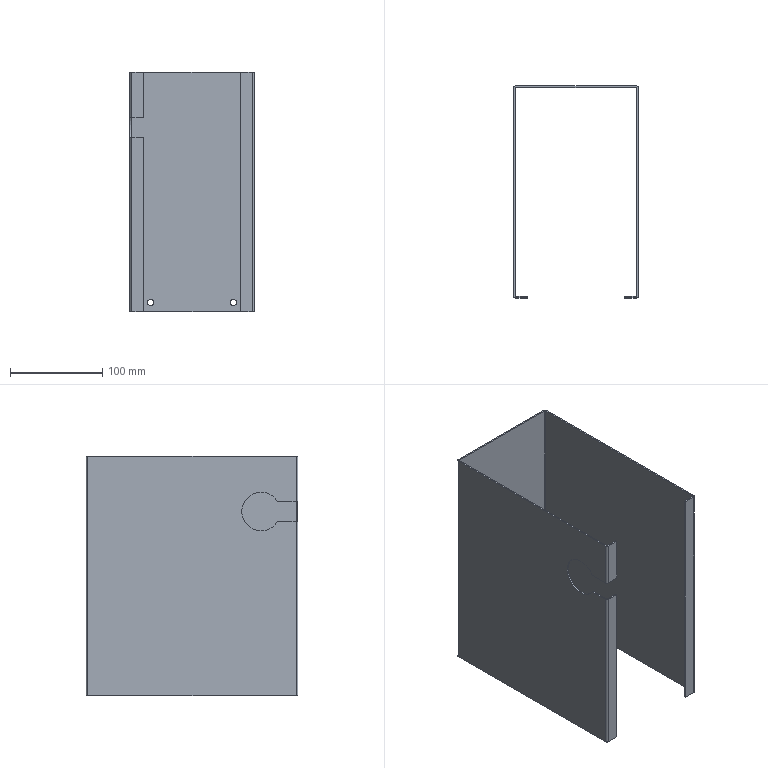Part | STEP file | X Motor Cover 1 | 1 solid | 36 faces | box 135 x 230 x 260 mm | volume 237291 mm3 | plane 19 | cylinder 17 | commonest cylinder face diameters 1 x5 4 x5 7 x4 42 x3
STEP:
#1=CARTESIAN_POINT('',(-74.708,228.5,-161.347));
#2=VERTEX_POINT('',#1);
#3=CARTESIAN_POINT('',(-74.708,228.5,-168.347));
#4=VERTEX_POINT('',#3);
#5=CARTESIAN_POINT('',(-74.708,228.5,-164.847));
#6=DIRECTION('',(0.,-1.,0.));
#7=DIRECTION('',(0.,0.,1.));
#8=AXIS2_PLACEMENT_3D('',#5,#6,#7);
#9=CIRCLE('',#8,3.5);
#10=EDGE_CURVE('',#2,#4,#9,.T.);
#11=ORIENTED_EDGE('',*,*,#10,.T.);
#12=CARTESIAN_POINT('',(-74.708,230.,-168.347));
#13=VERTEX_POINT('',#12);
#14=CARTESIAN_POINT('',(-74.708,208.,-168.347));
#15=DIRECTION('',(0.,1.,0.));
#16=VECTOR('',#15,1000.);
#17=LINE('',#14,#16);
#18=EDGE_CURVE('',#4,#13,#17,.T.);
#19=ORIENTED_EDGE('',*,*,#18,.T.);
#20=CARTESIAN_POINT('',(-74.708,230.,-161.347));
#21=VERTEX_POINT('',#20);
#22=CARTESIAN_POINT('',(-74.708,230.,-164.847));
#23=DIRECTION('',(0.,-1.,0.));
#24=DIRECTION('',(0.,0.,1.));
#25=AXIS2_PLACEMENT_3D('',#22,#23,#24);
#26=CIRCLE('',#25,3.5);
#27=EDGE_CURVE('',#21,#13,#26,.T.);
#28=ORIENTED_EDGE('',*,*,#27,.F.);
#29=CARTESIAN_POINT('',(-74.708,208.,-161.347));
#30=DIRECTION('',(0.,1.,0.));
#31=VECTOR('',#30,1000.);
#32=LINE('',#29,#31);
#33=EDGE_CURVE('',#2,#21,#32,.T.);
#34=ORIENTED_EDGE('',*,*,#33,.F.);
#35=EDGE_LOOP('',(#11,#19,#28,#34));
#36=FACE_OUTER_BOUND('',#35,.T.);
#37=CARTESIAN_POINT('',(-74.708,208.,-164.847));
#38=DIRECTION('',(0.,1.,0.));
#39=DIRECTION('',(0.,0.,1.));
#40=AXIS2_PLACEMENT_3D('',#37,#38,#39);
#41=CYLINDRICAL_SURFACE('',#40,3.5);
#42=ADVANCED_FACE('',(#36),#41,.F.);
#43=CARTESIAN_POINT('',(15.292,228.5,-161.347));
#44=VERTEX_POINT('',#43);
#45=CARTESIAN_POINT('',(15.292,228.5,-168.347));
#46=VERTEX_POINT('',#45);
#47=CARTESIAN_POINT('',(15.292,228.5,-164.847));
#48=DIRECTION('',(0.,-1.,0.));
#49=DIRECTION('',(0.,0.,1.));
#50=AXIS2_PLACEMENT_3D('',#47,#48,#49);
#51=CIRCLE('',#50,3.5);
#52=EDGE_CURVE('',#44,#46,#51,.T.);
#53=ORIENTED_EDGE('',*,*,#52,.T.);
#54=CARTESIAN_POINT('',(15.292,230.,-168.347));
#55=VERTEX_POINT('',#54);
#56=CARTESIAN_POINT('',(15.292,208.,-168.347));
#57=DIRECTION('',(0.,1.,0.));
#58=VECTOR('',#57,1000.);
#59=LINE('',#56,#58);
#60=EDGE_CURVE('',#46,#55,#59,.T.);
#61=ORIENTED_EDGE('',*,*,#60,.T.);
#62=CARTESIAN_POINT('',(15.292,230.,-161.347));
#63=VERTEX_POINT('',#62);
#64=CARTESIAN_POINT('',(15.292,230.,-164.847));
#65=DIRECTION('',(0.,-1.,0.));
#66=DIRECTION('',(0.,0.,1.));
#67=AXIS2_PLACEMENT_3D('',#64,#65,#66);
#68=CIRCLE('',#67,3.5);
#69=EDGE_CURVE('',#63,#55,#68,.T.);
#70=ORIENTED_EDGE('',*,*,#69,.F.);
#71=CARTESIAN_POINT('',(15.292,208.,-161.347));
#72=DIRECTION('',(0.,1.,0.));
#73=VECTOR('',#72,1000.);
#74=LINE('',#71,#73);
#75=EDGE_CURVE('',#44,#63,#74,.T.);
#76=ORIENTED_EDGE('',*,*,#75,.F.);
#77=EDGE_LOOP('',(#53,#61,#70,#76));
#78=FACE_OUTER_BOUND('',#77,.T.);
#79=CARTESIAN_POINT('',(15.292,208.,-164.847));
#80=DIRECTION('',(0.,1.,0.));
#81=DIRECTION('',(0.,0.,1.));
#82=AXIS2_PLACEMENT_3D('',#79,#80,#81);
#83=CYLINDRICAL_SURFACE('',#82,3.5);
#84=ADVANCED_FACE('',(#78),#83,.F.);
#85=CARTESIAN_POINT('',(-95.708,40.,4.153));
#86=VERTEX_POINT('',#85);
#87=CARTESIAN_POINT('',(-95.708,22.111,14.153));
#88=VERTEX_POINT('',#87);
#89=CARTESIAN_POINT('',(-95.708,40.,25.153));
#90=DIRECTION('',(-1.,0.,0.));
#91=DIRECTION('',(0.,0.,1.));
#92=AXIS2_PLACEMENT_3D('',#89,#90,#91);
#93=CIRCLE('',#92,21.);
#94=EDGE_CURVE('',#86,#88,#93,.T.);
#95=ORIENTED_EDGE('',*,*,#94,.F.);
#96=CARTESIAN_POINT('',(-97.208,40.,4.153));
#97=VERTEX_POINT('',#96);
#98=CARTESIAN_POINT('',(-75.208,40.,4.153));
#99=DIRECTION('',(-1.,0.,0.));
#100=VECTOR('',#99,1000.);
#101=LINE('',#98,#100);
#102=EDGE_CURVE('',#86,#97,#101,.T.);
#103=ORIENTED_EDGE('',*,*,#102,.T.);
#104=CARTESIAN_POINT('',(-97.208,22.111,14.153));
#105=VERTEX_POINT('',#104);
#106=CARTESIAN_POINT('',(-97.208,40.,25.153));
#107=DIRECTION('',(1.,0.,0.));
#108=DIRECTION('',(0.,0.,1.));
#109=AXIS2_PLACEMENT_3D('',#106,#107,#108);
#110=CIRCLE('',#109,21.);
#111=EDGE_CURVE('',#105,#97,#110,.T.);
#112=ORIENTED_EDGE('',*,*,#111,.F.);
#113=CARTESIAN_POINT('',(-75.208,22.111,14.153));
#114=DIRECTION('',(1.,0.,0.));
#115=VECTOR('',#114,1000.);
#116=LINE('',#113,#115);
#117=EDGE_CURVE('',#105,#88,#116,.T.);
#118=ORIENTED_EDGE('',*,*,#117,.T.);
#119=EDGE_LOOP('',(#95,#103,#112,#118));
#120=FACE_OUTER_BOUND('',#119,.T.);
#121=CARTESIAN_POINT('',(-75.208,40.,25.153));
#122=DIRECTION('',(-1.,0.,0.));
#123=DIRECTION('',(0.,0.,1.));
#124=AXIS2_PLACEMENT_3D('',#121,#122,#123);
#125=CYLINDRICAL_SURFACE('',#124,21.);
#126=ADVANCED_FACE('',(#120),#125,.F.);
#127=ORIENTED_EDGE('',*,*,#102,.F.);
#128=CARTESIAN_POINT('',(-95.708,40.,46.153));
#129=VERTEX_POINT('',#128);
#130=CARTESIAN_POINT('',(-95.708,40.,25.153));
#131=DIRECTION('',(-1.,0.,0.));
#132=DIRECTION('',(0.,0.,1.));
#133=AXIS2_PLACEMENT_3D('',#130,#131,#132);
#134=CIRCLE('',#133,21.);
#135=EDGE_CURVE('',#129,#86,#134,.T.);
#136=ORIENTED_EDGE('',*,*,#135,.F.);
#137=CARTESIAN_POINT('',(-97.208,40.,46.153));
#138=VERTEX_POINT('',#137);
#139=CARTESIAN_POINT('',(-75.208,40.,46.153));
#140=DIRECTION('',(-1.,0.,0.));
#141=VECTOR('',#140,1000.);
#142=LINE('',#139,#141);
#143=EDGE_CURVE('',#129,#138,#142,.T.);
#144=ORIENTED_EDGE('',*,*,#143,.T.);
#145=CARTESIAN_POINT('',(-97.208,40.,25.153));
#146=DIRECTION('',(1.,0.,0.));
#147=DIRECTION('',(0.,0.,1.));
#148=AXIS2_PLACEMENT_3D('',#145,#146,#147);
#149=CIRCLE('',#148,21.);
#150=EDGE_CURVE('',#97,#138,#149,.T.);
#151=ORIENTED_EDGE('',*,*,#150,.F.);
#152=EDGE_LOOP('',(#127,#136,#144,#151));
#153=FACE_OUTER_BOUND('',#152,.T.);
#154=CARTESIAN_POINT('',(-75.208,40.,25.153));
#155=DIRECTION('',(-1.,0.,0.));
#156=DIRECTION('',(0.,0.,1.));
#157=AXIS2_PLACEMENT_3D('',#154,#155,#156);
#158=CYLINDRICAL_SURFACE('',#157,21.);
#159=ADVANCED_FACE('',(#153),#158,.F.);
#160=CARTESIAN_POINT('',(36.292,2.,85.153));
#161=VERTEX_POINT('',#160);
#162=CARTESIAN_POINT('',(36.292,228.,85.153));
#163=VERTEX_POINT('',#162);
#164=CARTESIAN_POINT('',(36.292,230.,85.153));
#165=DIRECTION('',(0.,1.,0.));
#166=VECTOR('',#165,1000.);
#167=LINE('',#164,#166);
#168=EDGE_CURVE('',#161,#163,#167,.T.);
#169=ORIENTED_EDGE('',*,*,#168,.T.);
#170=CARTESIAN_POINT('',(36.292,228.,-174.847));
#171=VERTEX_POINT('',#170);
#172=CARTESIAN_POINT('',(36.292,228.,-174.847));
#173=DIRECTION('',(0.,0.,-1.));
#174=VECTOR('',#173,1000.);
#175=LINE('',#172,#174);
#176=EDGE_CURVE('',#163,#171,#175,.T.);
#177=ORIENTED_EDGE('',*,*,#176,.T.);
#178=CARTESIAN_POINT('',(36.292,2.,-174.847));
#179=VERTEX_POINT('',#178);
#180=CARTESIAN_POINT('',(36.292,230.,-174.847));
#181=DIRECTION('',(0.,-1.,0.));
#182=VECTOR('',#181,1000.);
#183=LINE('',#180,#182);
#184=EDGE_CURVE('',#171,#179,#183,.T.);
#185=ORIENTED_EDGE('',*,*,#184,.T.);
#186=CARTESIAN_POINT('',(36.292,2.,-174.847));
#187=DIRECTION('',(0.,0.,1.));
#188=VECTOR('',#187,1000.);
#189=LINE('',#186,#188);
#190=EDGE_CURVE('',#179,#161,#189,.T.);
#191=ORIENTED_EDGE('',*,*,#190,.T.);
#192=EDGE_LOOP('',(#169,#177,#185,#191));
#193=FACE_OUTER_BOUND('',#192,.T.);
#194=CARTESIAN_POINT('',(36.292,230.,-174.847));
#195=DIRECTION('',(-1.,0.,0.));
#196=DIRECTION('',(0.,0.,1.));
#197=AXIS2_PLACEMENT_3D('',#194,#195,#196);
#198=PLANE('',#197);
#199=ADVANCED_FACE('',(#193),#198,.T.);
#200=CARTESIAN_POINT('',(35.792,228.5,-174.847));
#201=VERTEX_POINT('',#200);
#202=CARTESIAN_POINT('',(35.792,228.,-174.847));
#203=DIRECTION('',(0.,0.,1.));
#204=DIRECTION('',(1.,0.,0.));
#205=AXIS2_PLACEMENT_3D('',#202,#203,#204);
#206=CIRCLE('',#205,0.5);
#207=EDGE_CURVE('',#171,#201,#206,.T.);
#208=ORIENTED_EDGE('',*,*,#207,.F.);
#209=ORIENTED_EDGE('',*,*,#176,.F.);
#210=CARTESIAN_POINT('',(35.792,228.5,85.153));
#211=VERTEX_POINT('',#210);
#212=CARTESIAN_POINT('',(35.792,228.,85.153));
#213=DIRECTION('',(0.,0.,-1.));
#214=DIRECTION('',(1.,0.,0.));
#215=AXIS2_PLACEMENT_3D('',#212,#213,#214);
#216=CIRCLE('',#215,0.5);
#217=EDGE_CURVE('',#211,#163,#216,.T.);
#218=ORIENTED_EDGE('',*,*,#217,.F.);
#219=CARTESIAN_POINT('',(35.792,228.5,-842.522));
#220=DIRECTION('',(0.,0.,1.));
#221=VECTOR('',#220,1000.);
#222=LINE('',#219,#221);
#223=EDGE_CURVE('',#201,#211,#222,.T.);
#224=ORIENTED_EDGE('',*,*,#223,.F.);
#225=EDGE_LOOP('',(#208,#209,#218,#224));
#226=FACE_OUTER_BOUND('',#225,.T.);
#227=CARTESIAN_POINT('',(35.792,228.,-842.522));
#228=DIRECTION('',(0.,0.,1.));
#229=DIRECTION('',(1.,0.,0.));
#230=AXIS2_PLACEMENT_3D('',#227,#228,#229);
#231=CYLINDRICAL_SURFACE('',#230,0.5);
#232=ADVANCED_FACE('',(#226),#231,.F.);
#233=ORIENTED_EDGE('',*,*,#168,.F.);
#234=CARTESIAN_POINT('',(35.792,1.5,85.153));
#235=VERTEX_POINT('',#234);
#236=CARTESIAN_POINT('',(35.792,2.,85.153));
#237=DIRECTION('',(0.,0.,-1.));
#238=DIRECTION('',(1.,0.,0.));
#239=AXIS2_PLACEMENT_3D('',#236,#237,#238);
#240=CIRCLE('',#239,0.5);
#241=EDGE_CURVE('',#161,#235,#240,.T.);
#242=ORIENTED_EDGE('',*,*,#241,.T.);
#243=CARTESIAN_POINT('',(22.792,1.5,85.153));
#244=VERTEX_POINT('',#243);
#245=CARTESIAN_POINT('',(0.,1.5,85.153));
#246=DIRECTION('',(1.,0.,0.));
#247=VECTOR('',#246,1000.);
#248=LINE('',#245,#247);
#249=EDGE_CURVE('',#244,#235,#248,.T.);
#250=ORIENTED_EDGE('',*,*,#249,.F.);
#251=CARTESIAN_POINT('',(22.792,0.,85.153));
#252=VERTEX_POINT('',#251);
#253=CARTESIAN_POINT('',(22.792,522.15,85.153));
#254=DIRECTION('',(0.,1.,0.));
#255=VECTOR('',#254,1000.);
#256=LINE('',#253,#255);
#257=EDGE_CURVE('',#252,#244,#256,.T.);
#258=ORIENTED_EDGE('',*,*,#257,.F.);
#259=CARTESIAN_POINT('',(35.792,0.,85.153));
#260=VERTEX_POINT('',#259);
#261=CARTESIAN_POINT('',(-97.208,0.,85.153));
#262=DIRECTION('',(-1.,0.,0.));
#263=VECTOR('',#262,1000.);
#264=LINE('',#261,#263);
#265=EDGE_CURVE('',#260,#252,#264,.T.);
#266=ORIENTED_EDGE('',*,*,#265,.F.);
#267=CARTESIAN_POINT('',(37.792,2.,85.153));
#268=VERTEX_POINT('',#267);
#269=CARTESIAN_POINT('',(35.792,2.,85.153));
#270=DIRECTION('',(0.,0.,-1.));
#271=DIRECTION('',(1.,0.,0.));
#272=AXIS2_PLACEMENT_3D('',#269,#270,#271);
#273=CIRCLE('',#272,2.);
#274=EDGE_CURVE('',#268,#260,#273,.T.);
#275=ORIENTED_EDGE('',*,*,#274,.F.);
#276=CARTESIAN_POINT('',(37.792,228.,85.153));
#277=VERTEX_POINT('',#276);
#278=CARTESIAN_POINT('',(37.792,230.,85.153));
#279=DIRECTION('',(0.,1.,0.));
#280=VECTOR('',#279,1000.);
#281=LINE('',#278,#280);
#282=EDGE_CURVE('',#268,#277,#281,.T.);
#283=ORIENTED_EDGE('',*,*,#282,.T.);
#284=CARTESIAN_POINT('',(35.792,230.,85.153));
#285=VERTEX_POINT('',#284);
#286=CARTESIAN_POINT('',(35.792,228.,85.153));
#287=DIRECTION('',(0.,0.,-1.));
#288=DIRECTION('',(1.,0.,0.));
#289=AXIS2_PLACEMENT_3D('',#286,#287,#288);
#290=CIRCLE('',#289,2.);
#291=EDGE_CURVE('',#285,#277,#290,.T.);
#292=ORIENTED_EDGE('',*,*,#291,.F.);
#293=CARTESIAN_POINT('',(-95.208,230.,85.153));
#294=VERTEX_POINT('',#293);
#295=CARTESIAN_POINT('',(-97.208,230.,85.153));
#296=DIRECTION('',(-1.,0.,0.));
#297=VECTOR('',#296,1000.);
#298=LINE('',#295,#297);
#299=EDGE_CURVE('',#285,#294,#298,.T.);
#300=ORIENTED_EDGE('',*,*,#299,.T.);
#301=CARTESIAN_POINT('',(-97.208,228.,85.153));
#302=VERTEX_POINT('',#301);
#303=CARTESIAN_POINT('',(-95.208,228.,85.153));
#304=DIRECTION('',(0.,0.,-1.));
#305=DIRECTION('',(-1.,0.,0.));
#306=AXIS2_PLACEMENT_3D('',#303,#304,#305);
#307=CIRCLE('',#306,2.);
#308=EDGE_CURVE('',#302,#294,#307,.T.);
#309=ORIENTED_EDGE('',*,*,#308,.F.);
#310=CARTESIAN_POINT('',(-97.208,2.,85.153));
#311=VERTEX_POINT('',#310);
#312=CARTESIAN_POINT('',(-97.208,230.,85.153));
#313=DIRECTION('',(0.,1.,0.));
#314=VECTOR('',#313,1000.);
#315=LINE('',#312,#314);
#316=EDGE_CURVE('',#311,#302,#315,.T.);
#317=ORIENTED_EDGE('',*,*,#316,.F.);
#318=CARTESIAN_POINT('',(-95.208,0.,85.153));
#319=VERTEX_POINT('',#318);
#320=CARTESIAN_POINT('',(-95.208,2.,85.153));
#321=DIRECTION('',(0.,0.,-1.));
#322=DIRECTION('',(-1.,0.,0.));
#323=AXIS2_PLACEMENT_3D('',#320,#321,#322);
#324=CIRCLE('',#323,2.);
#325=EDGE_CURVE('',#319,#311,#324,.T.);
#326=ORIENTED_EDGE('',*,*,#325,.F.);
#327=CARTESIAN_POINT('',(-82.208,0.,85.153));
#328=VERTEX_POINT('',#327);
#329=CARTESIAN_POINT('',(0.,0.,85.153));
#330=DIRECTION('',(1.,0.,0.));
#331=VECTOR('',#330,1000.);
#332=LINE('',#329,#331);
#333=EDGE_CURVE('',#319,#328,#332,.T.);
#334=ORIENTED_EDGE('',*,*,#333,.T.);
#335=CARTESIAN_POINT('',(-82.208,1.5,85.153));
#336=VERTEX_POINT('',#335);
#337=CARTESIAN_POINT('',(-82.208,522.15,85.153));
#338=DIRECTION('',(0.,1.,0.));
#339=VECTOR('',#338,1000.);
#340=LINE('',#337,#339);
#341=EDGE_CURVE('',#328,#336,#340,.T.);
#342=ORIENTED_EDGE('',*,*,#341,.T.);
#343=CARTESIAN_POINT('',(-95.208,1.5,85.153));
#344=VERTEX_POINT('',#343);
#345=CARTESIAN_POINT('',(0.,1.5,85.153));
#346=DIRECTION('',(1.,0.,0.));
#347=VECTOR('',#346,1000.);
#348=LINE('',#345,#347);
#349=EDGE_CURVE('',#344,#336,#348,.T.);
#350=ORIENTED_EDGE('',*,*,#349,.F.);
#351=CARTESIAN_POINT('',(-95.708,2.,85.153));
#352=VERTEX_POINT('',#351);
#353=CARTESIAN_POINT('',(-95.208,2.,85.153));
#354=DIRECTION('',(0.,0.,-1.));
#355=DIRECTION('',(-1.,0.,0.));
#356=AXIS2_PLACEMENT_3D('',#353,#354,#355);
#357=CIRCLE('',#356,0.5);
#358=EDGE_CURVE('',#344,#352,#357,.T.);
#359=ORIENTED_EDGE('',*,*,#358,.T.);
#360=CARTESIAN_POINT('',(-95.708,228.,85.153));
#361=VERTEX_POINT('',#360);
#362=CARTESIAN_POINT('',(-95.708,230.,85.153));
#363=DIRECTION('',(0.,-1.,0.));
#364=VECTOR('',#363,1000.);
#365=LINE('',#362,#364);
#366=EDGE_CURVE('',#361,#352,#365,.T.);
#367=ORIENTED_EDGE('',*,*,#366,.F.);
#368=CARTESIAN_POINT('',(-95.208,228.5,85.153));
#369=VERTEX_POINT('',#368);
#370=CARTESIAN_POINT('',(-95.208,228.,85.153));
#371=DIRECTION('',(0.,0.,-1.));
#372=DIRECTION('',(-1.,0.,0.));
#373=AXIS2_PLACEMENT_3D('',#370,#371,#372);
#374=CIRCLE('',#373,0.5);
#375=EDGE_CURVE('',#361,#369,#374,.T.);
#376=ORIENTED_EDGE('',*,*,#375,.T.);
#377=CARTESIAN_POINT('',(0.,228.5,85.153));
#378=DIRECTION('',(1.,0.,0.));
#379=VECTOR('',#378,1000.);
#380=LINE('',#377,#379);
#381=EDGE_CURVE('',#369,#211,#380,.T.);
#382=ORIENTED_EDGE('',*,*,#381,.T.);
#383=ORIENTED_EDGE('',*,*,#217,.T.);
#384=EDGE_LOOP('',(#233,#242,#250,#258,#266,#275,#283,#292,#300,#309,#317,#326,#334,#342,#350,#359,#367,#376,#382,#383));
#385=FACE_OUTER_BOUND('',#384,.T.);
#386=CARTESIAN_POINT('',(-652.695,230.,85.153));
#387=DIRECTION('',(0.,0.,1.));
#388=DIRECTION('',(1.,0.,0.));
#389=AXIS2_PLACEMENT_3D('',#386,#387,#388);
#390=PLANE('',#389);
#391=ADVANCED_FACE('',(#385),#390,.T.);
#392=CARTESIAN_POINT('',(35.792,1.5,-174.847));
#393=VERTEX_POINT('',#392);
#394=CARTESIAN_POINT('',(35.792,1.5,-555.146));
#395=DIRECTION('',(0.,0.,-1.));
#396=VECTOR('',#395,1000.);
#397=LINE('',#394,#396);
#398=EDGE_CURVE('',#235,#393,#397,.T.);
#399=ORIENTED_EDGE('',*,*,#398,.F.);
#400=ORIENTED_EDGE('',*,*,#241,.F.);
#401=ORIENTED_EDGE('',*,*,#190,.F.);
#402=CARTESIAN_POINT('',(35.792,2.,-174.847));
#403=DIRECTION('',(0.,0.,1.));
#404=DIRECTION('',(1.,0.,0.));
#405=AXIS2_PLACEMENT_3D('',#402,#403,#404);
#406=CIRCLE('',#405,0.5);
#407=EDGE_CURVE('',#393,#179,#406,.T.);
#408=ORIENTED_EDGE('',*,*,#407,.F.);
#409=EDGE_LOOP('',(#399,#400,#401,#408));
#410=FACE_OUTER_BOUND('',#409,.T.);
#411=CARTESIAN_POINT('',(35.792,2.,-555.146));
#412=DIRECTION('',(0.,0.,1.));
#413=DIRECTION('',(1.,0.,0.));
#414=AXIS2_PLACEMENT_3D('',#411,#412,#413);
#415=CYLINDRICAL_SURFACE('',#414,0.5);
#416=ADVANCED_FACE('',(#410),#415,.F.);
#417=CARTESIAN_POINT('',(37.792,2.,-174.847));
#418=VERTEX_POINT('',#417);
#419=CARTESIAN_POINT('',(37.792,228.,-174.847));
#420=VERTEX_POINT('',#419);
#421=CARTESIAN_POINT('',(37.792,230.,-174.847));
#422=DIRECTION('',(0.,1.,0.));
#423=VECTOR('',#422,1000.);
#424=LINE('',#421,#423);
#425=EDGE_CURVE('',#418,#420,#424,.T.);
#426=ORIENTED_EDGE('',*,*,#425,.F.);
#427=CARTESIAN_POINT('',(35.792,0.,-174.847));
#428=VERTEX_POINT('',#427);
#429=CARTESIAN_POINT('',(35.792,2.,-174.847));
#430=DIRECTION('',(0.,0.,1.));
#431=DIRECTION('',(1.,0.,0.));
#432=AXIS2_PLACEMENT_3D('',#429,#430,#431);
#433=CIRCLE('',#432,2.);
#434=EDGE_CURVE('',#428,#418,#433,.T.);
#435=ORIENTED_EDGE('',*,*,#434,.F.);
#436=CARTESIAN_POINT('',(22.792,0.,-174.847));
#437=VERTEX_POINT('',#436);
#438=CARTESIAN_POINT('',(-97.208,0.,-174.847));
#439=DIRECTION('',(1.,0.,0.));
#440=VECTOR('',#439,1000.);
#441=LINE('',#438,#440);
#442=EDGE_CURVE('',#437,#428,#441,.T.);
#443=ORIENTED_EDGE('',*,*,#442,.F.);
#444=CARTESIAN_POINT('',(22.792,1.5,-174.847));
#445=VERTEX_POINT('',#444);
#446=CARTESIAN_POINT('',(22.792,522.15,-174.847));
#447=DIRECTION('',(0.,1.,0.));
#448=VECTOR('',#447,1000.);
#449=LINE('',#446,#448);
#450=EDGE_CURVE('',#437,#445,#449,.T.);
#451=ORIENTED_EDGE('',*,*,#450,.T.);
#452=CARTESIAN_POINT('',(0.,1.5,-174.847));
#453=DIRECTION('',(-1.,0.,0.));
#454=VECTOR('',#453,1000.);
#455=LINE('',#452,#454);
#456=EDGE_CURVE('',#393,#445,#455,.T.);
#457=ORIENTED_EDGE('',*,*,#456,.F.);
#458=ORIENTED_EDGE('',*,*,#407,.T.);
#459=ORIENTED_EDGE('',*,*,#184,.F.);
#460=ORIENTED_EDGE('',*,*,#207,.T.);
#461=CARTESIAN_POINT('',(-95.208,228.5,-174.847));
#462=VERTEX_POINT('',#461);
#463=CARTESIAN_POINT('',(0.,228.5,-174.847));
#464=DIRECTION('',(-1.,0.,0.));
#465=VECTOR('',#464,1000.);
#466=LINE('',#463,#465);
#467=EDGE_CURVE('',#201,#462,#466,.T.);
#468=ORIENTED_EDGE('',*,*,#467,.T.);
#469=CARTESIAN_POINT('',(-95.708,228.,-174.847));
#470=VERTEX_POINT('',#469);
#471=CARTESIAN_POINT('',(-95.208,228.,-174.847));
#472=DIRECTION('',(0.,0.,1.));
#473=DIRECTION('',(-1.,0.,0.));
#474=AXIS2_PLACEMENT_3D('',#471,#472,#473);
#475=CIRCLE('',#474,0.5);
#476=EDGE_CURVE('',#462,#470,#475,.T.);
#477=ORIENTED_EDGE('',*,*,#476,.T.);
#478=CARTESIAN_POINT('',(-95.708,2.,-174.847));
#479=VERTEX_POINT('',#478);
#480=CARTESIAN_POINT('',(-95.708,230.,-174.847));
#481=DIRECTION('',(0.,1.,0.));
#482=VECTOR('',#481,1000.);
#483=LINE('',#480,#482);
#484=EDGE_CURVE('',#479,#470,#483,.T.);
#485=ORIENTED_EDGE('',*,*,#484,.F.);
#486=CARTESIAN_POINT('',(-95.208,1.5,-174.847));
#487=VERTEX_POINT('',#486);
#488=CARTESIAN_POINT('',(-95.208,2.,-174.847));
#489=DIRECTION('',(0.,0.,1.));
#490=DIRECTION('',(-1.,0.,0.));
#491=AXIS2_PLACEMENT_3D('',#488,#489,#490);
#492=CIRCLE('',#491,0.5);
#493=EDGE_CURVE('',#479,#487,#492,.T.);
#494=ORIENTED_EDGE('',*,*,#493,.T.);
#495=CARTESIAN_POINT('',(-82.208,1.5,-174.847));
#496=VERTEX_POINT('',#495);
#497=CARTESIAN_POINT('',(0.,1.5,-174.847));
#498=DIRECTION('',(-1.,0.,0.));
#499=VECTOR('',#498,1000.);
#500=LINE('',#497,#499);
#501=EDGE_CURVE('',#496,#487,#500,.T.);
#502=ORIENTED_EDGE('',*,*,#501,.F.);
#503=CARTESIAN_POINT('',(-82.208,0.,-174.847));
#504=VERTEX_POINT('',#503);
#505=CARTESIAN_POINT('',(-82.208,522.15,-174.847));
#506=DIRECTION('',(0.,1.,0.));
#507=VECTOR('',#506,1000.);
#508=LINE('',#505,#507);
#509=EDGE_CURVE('',#504,#496,#508,.T.);
#510=ORIENTED_EDGE('',*,*,#509,.F.);
#511=CARTESIAN_POINT('',(-95.208,0.,-174.847));
#512=VERTEX_POINT('',#511);
#513=CARTESIAN_POINT('',(0.,0.,-174.847));
#514=DIRECTION('',(-1.,0.,0.));
#515=VECTOR('',#514,1000.);
#516=LINE('',#513,#515);
#517=EDGE_CURVE('',#504,#512,#516,.T.);
#518=ORIENTED_EDGE('',*,*,#517,.T.);
#519=CARTESIAN_POINT('',(-97.208,2.,-174.847));
#520=VERTEX_POINT('',#519);
#521=CARTESIAN_POINT('',(-95.208,2.,-174.847));
#522=DIRECTION('',(0.,0.,1.));
#523=DIRECTION('',(-1.,0.,0.));
#524=AXIS2_PLACEMENT_3D('',#521,#522,#523);
#525=CIRCLE('',#524,2.);
#526=EDGE_CURVE('',#520,#512,#525,.T.);
#527=ORIENTED_EDGE('',*,*,#526,.F.);
#528=CARTESIAN_POINT('',(-97.208,228.,-174.847));
#529=VERTEX_POINT('',#528);
#530=CARTESIAN_POINT('',(-97.208,230.,-174.847));
#531=DIRECTION('',(0.,1.,0.));
#532=VECTOR('',#531,1000.);
#533=LINE('',#530,#532);
#534=EDGE_CURVE('',#520,#529,#533,.T.);
#535=ORIENTED_EDGE('',*,*,#534,.T.);
#536=CARTESIAN_POINT('',(-95.208,230.,-174.847));
#537=VERTEX_POINT('',#536);
#538=CARTESIAN_POINT('',(-95.208,228.,-174.847));
#539=DIRECTION('',(0.,0.,1.));
#540=DIRECTION('',(-1.,0.,0.));
#541=AXIS2_PLACEMENT_3D('',#538,#539,#540);
#542=CIRCLE('',#541,2.);
#543=EDGE_CURVE('',#537,#529,#542,.T.);
#544=ORIENTED_EDGE('',*,*,#543,.F.);
#545=CARTESIAN_POINT('',(35.792,230.,-174.847));
#546=VERTEX_POINT('',#545);
#547=CARTESIAN_POINT('',(-97.208,230.,-174.847));
#548=DIRECTION('',(1.,0.,0.));
#549=VECTOR('',#548,1000.);
#550=LINE('',#547,#549);
#551=EDGE_CURVE('',#537,#546,#550,.T.);
#552=ORIENTED_EDGE('',*,*,#551,.T.);
#553=CARTESIAN_POINT('',(35.792,228.,-174.847));
#554=DIRECTION('',(0.,0.,1.));
#555=DIRECTION('',(1.,0.,0.));
#556=AXIS2_PLACEMENT_3D('',#553,#554,#555);
#557=CIRCLE('',#556,2.);
#558=EDGE_CURVE('',#420,#546,#557,.T.);
#559=ORIENTED_EDGE('',*,*,#558,.F.);
#560=EDGE_LOOP('',(#426,#435,#443,#451,#457,#458,#459,#460,#468,#477,#485,#494,#502,#510,#518,#527,#535,#544,#552,#559));
#561=FACE_OUTER_BOUND('',#560,.T.);
#562=CARTESIAN_POINT('',(-652.695,230.,-174.847));
#563=DIRECTION('',(0.,0.,1.));
#564=DIRECTION('',(1.,0.,0.));
#565=AXIS2_PLACEMENT_3D('',#562,#563,#564);
#566=PLANE('',#565);
#567=ADVANCED_FACE('',(#561),#566,.F.);
#568=ORIENTED_EDGE('',*,*,#467,.F.);
#569=ORIENTED_EDGE('',*,*,#223,.T.);
#570=ORIENTED_EDGE('',*,*,#381,.F.);
#571=CARTESIAN_POINT('',(-95.208,228.5,0.));
#572=DIRECTION('',(0.,0.,1.));
#573=VECTOR('',#572,1000.);
#574=LINE('',#571,#573);
#575=EDGE_CURVE('',#462,#369,#574,.T.);
#576=ORIENTED_EDGE('',*,*,#575,.F.);
#577=EDGE_LOOP('',(#568,#569,#570,#576));
#578=FACE_OUTER_BOUND('',#577,.T.);
#579=ORIENTED_EDGE('',*,*,#10,.F.);
#580=CARTESIAN_POINT('',(-74.708,228.5,-164.847));
#581=DIRECTION('',(0.,-1.,0.));
#582=DIRECTION('',(0.,0.,1.));
#583=AXIS2_PLACEMENT_3D('',#580,#581,#582);
#584=CIRCLE('',#583,3.5);
#585=EDGE_CURVE('',#4,#2,#584,.T.);
#586=ORIENTED_EDGE('',*,*,#585,.F.);
#587=EDGE_LOOP('',(#579,#586));
#588=FACE_BOUND('',#587,.T.);
#589=ORIENTED_EDGE('',*,*,#52,.F.);
#590=CARTESIAN_POINT('',(15.292,228.5,-164.847));
#591=DIRECTION('',(0.,-1.,0.));
#592=DIRECTION('',(0.,0.,1.));
#593=AXIS2_PLACEMENT_3D('',#590,#591,#592);
#594=CIRCLE('',#593,3.5);
#595=EDGE_CURVE('',#46,#44,#594,.T.);
#596=ORIENTED_EDGE('',*,*,#595,.F.);
#597=EDGE_LOOP('',(#589,#596));
#598=FACE_BOUND('',#597,.T.);
#599=CARTESIAN_POINT('',(0.,228.5,0.));
#600=DIRECTION('',(0.,1.,0.));
#601=DIRECTION('',(0.,0.,1.));
#602=AXIS2_PLACEMENT_3D('',#599,#600,#601);
#603=PLANE('',#602);
#604=ADVANCED_FACE('',(#578,#588,#598),#603,.F.);
#605=ORIENTED_EDGE('',*,*,#425,.T.);
#606=CARTESIAN_POINT('',(37.792,228.,-174.847));
#607=DIRECTION('',(0.,0.,-1.));
#608=VECTOR('',#607,1000.);
#609=LINE('',#606,#608);
#610=EDGE_CURVE('',#277,#420,#609,.T.);
#611=ORIENTED_EDGE('',*,*,#610,.F.);
#612=ORIENTED_EDGE('',*,*,#282,.F.);
#613=CARTESIAN_POINT('',(37.792,2.,-174.847));
#614=DIRECTION('',(0.,0.,1.));
#615=VECTOR('',#614,1000.);
#616=LINE('',#613,#615);
#617=EDGE_CURVE('',#418,#268,#616,.T.);
#618=ORIENTED_EDGE('',*,*,#617,.F.);
#619=EDGE_LOOP('',(#605,#611,#612,#618));
#620=FACE_OUTER_BOUND('',#619,.T.);
#621=CARTESIAN_POINT('',(37.792,230.,-174.847));
#622=DIRECTION('',(-1.,0.,0.));
#623=DIRECTION('',(0.,0.,1.));
#624=AXIS2_PLACEMENT_3D('',#621,#622,#623);
#625=PLANE('',#624);
#626=ADVANCED_FACE('',(#620),#625,.F.);
#627=CARTESIAN_POINT('',(22.792,1.5,0.));
#628=DIRECTION('',(0.,0.,1.));
#629=VECTOR('',#628,1000.);
#630=LINE('',#627,#629);
#631=EDGE_CURVE('',#445,#244,#630,.T.);
#632=ORIENTED_EDGE('',*,*,#631,.T.);
#633=ORIENTED_EDGE('',*,*,#249,.T.);
#634=ORIENTED_EDGE('',*,*,#398,.T.);
#635=ORIENTED_EDGE('',*,*,#456,.T.);
#636=EDGE_LOOP('',(#632,#633,#634,#635));
#637=FACE_OUTER_BOUND('',#636,.T.);
#638=CARTESIAN_POINT('',(0.,1.5,0.));
#639=DIRECTION('',(0.,1.,0.));
#640=DIRECTION('',(0.,0.,1.));
#641=AXIS2_PLACEMENT_3D('',#638,#639,#640);
#642=PLANE('',#641);
#643=ADVANCED_FACE('',(#637),#642,.T.);
#644=ORIENTED_EDGE('',*,*,#375,.F.);
#645=CARTESIAN_POINT('',(-95.708,228.,601.889));
#646=DIRECTION('',(0.,0.,1.));
#647=VECTOR('',#646,1000.);
#648=LINE('',#645,#647);
#649=EDGE_CURVE('',#470,#361,#648,.T.);
#650=ORIENTED_EDGE('',*,*,#649,.F.);
#651=ORIENTED_EDGE('',*,*,#476,.F.);
#652=ORIENTED_EDGE('',*,*,#575,.T.);
#653=EDGE_LOOP('',(#644,#650,#651,#652));
#654=FACE_OUTER_BOUND('',#653,.T.);
#655=CARTESIAN_POINT('',(-95.208,228.,601.889));
#656=DIRECTION('',(0.,0.,-1.));
#657=DIRECTION('',(-1.,0.,0.));
#658=AXIS2_PLACEMENT_3D('',#655,#656,#657);
#659=CYLINDRICAL_SURFACE('',#658,0.5);
#660=ADVANCED_FACE('',(#654),#659,.F.);
#661=ORIENTED_EDGE('',*,*,#18,.F.);
#662=ORIENTED_EDGE('',*,*,#585,.T.);
#663=ORIENTED_EDGE('',*,*,#33,.T.);
#664=CARTESIAN_POINT('',(-74.708,230.,-164.847));
#665=DIRECTION('',(0.,-1.,0.));
#666=DIRECTION('',(0.,0.,1.));
#667=AXIS2_PLACEMENT_3D('',#664,#665,#666);
#668=CIRCLE('',#667,3.5);
#669=EDGE_CURVE('',#13,#21,#668,.T.);
#670=ORIENTED_EDGE('',*,*,#669,.F.);
#671=EDGE_LOOP('',(#661,#662,#663,#670));
#672=FACE_OUTER_BOUND('',#671,.T.);
#673=CARTESIAN_POINT('',(-74.708,208.,-164.847));
#674=DIRECTION('',(0.,1.,0.));
#675=DIRECTION('',(0.,0.,1.));
#676=AXIS2_PLACEMENT_3D('',#673,#674,#675);
#677=CYLINDRICAL_SURFACE('',#676,3.5);
#678=ADVANCED_FACE('',(#672),#677,.F.);
#679=ORIENTED_EDGE('',*,*,#60,.F.);
#680=ORIENTED_EDGE('',*,*,#595,.T.);
#681=ORIENTED_EDGE('',*,*,#75,.T.);
#682=CARTESIAN_POINT('',(15.292,230.,-164.847));
#683=DIRECTION('',(0.,-1.,0.));
#684=DIRECTION('',(0.,0.,1.));
#685=AXIS2_PLACEMENT_3D('',#682,#683,#684);
#686=CIRCLE('',#685,3.5);
#687=EDGE_CURVE('',#55,#63,#686,.T.);
#688=ORIENTED_EDGE('',*,*,#687,.F.);
#689=EDGE_LOOP('',(#679,#680,#681,#688));
#690=FACE_OUTER_BOUND('',#689,.T.);
#691=CARTESIAN_POINT('',(15.292,208.,-164.847));
#692=DIRECTION('',(0.,1.,0.));
#693=DIRECTION('',(0.,0.,1.));
#694=AXIS2_PLACEMENT_3D('',#691,#692,#693);
#695=CYLINDRICAL_SURFACE('',#694,3.5);
#696=ADVANCED_FACE('',(#690),#695,.F.);
#697=ORIENTED_EDGE('',*,*,#274,.T.);
#698=CARTESIAN_POINT('',(35.792,0.,-555.146));
#699=DIRECTION('',(0.,0.,-1.));
#700=VECTOR('',#699,1000.);
#701=LINE('',#698,#700);
#702=EDGE_CURVE('',#260,#428,#701,.T.);
#703=ORIENTED_EDGE('',*,*,#702,.T.);
#704=ORIENTED_EDGE('',*,*,#434,.T.);
#705=ORIENTED_EDGE('',*,*,#617,.T.);
#706=EDGE_LOOP('',(#697,#703,#704,#705));
#707=FACE_OUTER_BOUND('',#706,.T.);
#708=CARTESIAN_POINT('',(35.792,2.,-555.146));
#709=DIRECTION('',(0.,0.,1.));
#710=DIRECTION('',(1.,0.,0.));
#711=AXIS2_PLACEMENT_3D('',#708,#709,#710);
#712=CYLINDRICAL_SURFACE('',#711,2.);
#713=ADVANCED_FACE('',(#707),#712,.T.);
#714=ORIENTED_EDGE('',*,*,#610,.T.);
#715=ORIENTED_EDGE('',*,*,#558,.T.);
#716=CARTESIAN_POINT('',(35.792,230.,-842.522));
#717=DIRECTION('',(0.,0.,1.));
#718=VECTOR('',#717,1000.);
#719=LINE('',#716,#718);
#720=EDGE_CURVE('',#546,#285,#719,.T.);
#721=ORIENTED_EDGE('',*,*,#720,.T.);
#722=ORIENTED_EDGE('',*,*,#291,.T.);
#723=EDGE_LOOP('',(#714,#715,#721,#722));
#724=FACE_OUTER_BOUND('',#723,.T.);
#725=CARTESIAN_POINT('',(35.792,228.,-842.522));
#726=DIRECTION('',(0.,0.,1.));
#727=DIRECTION('',(1.,0.,0.));
#728=AXIS2_PLACEMENT_3D('',#725,#726,#727);
#729=CYLINDRICAL_SURFACE('',#728,2.);
#730=ADVANCED_FACE('',(#724),#729,.T.);
#731=CARTESIAN_POINT('',(22.792,0.,85.153));
#732=DIRECTION('',(0.,0.,-1.));
#733=VECTOR('',#732,1000.);
#734=LINE('',#731,#733);
#735=EDGE_CURVE('',#252,#437,#734,.T.);
#736=ORIENTED_EDGE('',*,*,#735,.F.);
#737=ORIENTED_EDGE('',*,*,#257,.T.);
#738=ORIENTED_EDGE('',*,*,#631,.F.);
#739=ORIENTED_EDGE('',*,*,#450,.F.);
#740=EDGE_LOOP('',(#736,#737,#738,#739));
#741=FACE_OUTER_BOUND('',#740,.T.);
#742=CARTESIAN_POINT('',(22.792,522.15,85.153));
#743=DIRECTION('',(1.,0.,0.));
#744=DIRECTION('',(0.,0.,-1.));
#745=AXIS2_PLACEMENT_3D('',#742,#743,#744);
#746=PLANE('',#745);
#747=ADVANCED_FACE('',(#741),#746,.F.);
#748=ORIENTED_EDGE('',*,*,#366,.T.);
#749=CARTESIAN_POINT('',(-95.708,2.,36.153));
#750=VERTEX_POINT('',#749);
#751=CARTESIAN_POINT('',(-95.708,2.,-174.847));
#752=DIRECTION('',(0.,0.,-1.));
#753=VECTOR('',#752,1000.);
#754=LINE('',#751,#753);
#755=EDGE_CURVE('',#352,#750,#754,.T.);
#756=ORIENTED_EDGE('',*,*,#755,.T.);
#757=CARTESIAN_POINT('',(-95.708,22.111,36.153));
#758=VERTEX_POINT('',#757);
#759=CARTESIAN_POINT('',(-95.708,230.,36.153));
#760=DIRECTION('',(0.,1.,0.));
#761=VECTOR('',#760,1000.);
#762=LINE('',#759,#761);
#763=EDGE_CURVE('',#750,#758,#762,.T.);
#764=ORIENTED_EDGE('',*,*,#763,.T.);
#765=CARTESIAN_POINT('',(-95.708,40.,25.153));
#766=DIRECTION('',(-1.,0.,0.));
#767=DIRECTION('',(0.,0.,1.));
#768=AXIS2_PLACEMENT_3D('',#765,#766,#767);
#769=CIRCLE('',#768,21.);
#770=EDGE_CURVE('',#758,#129,#769,.T.);
#771=ORIENTED_EDGE('',*,*,#770,.T.);
#772=ORIENTED_EDGE('',*,*,#135,.T.);
#773=ORIENTED_EDGE('',*,*,#94,.T.);
#774=CARTESIAN_POINT('',(-95.708,2.,14.153));
#775=VERTEX_POINT('',#774);
#776=CARTESIAN_POINT('',(-95.708,230.,14.153));
#777=DIRECTION('',(0.,-1.,0.));
#778=VECTOR('',#777,1000.);
#779=LINE('',#776,#778);
#780=EDGE_CURVE('',#88,#775,#779,.T.);
#781=ORIENTED_EDGE('',*,*,#780,.T.);
#782=CARTESIAN_POINT('',(-95.708,2.,-174.847));
#783=DIRECTION('',(0.,0.,-1.));
#784=VECTOR('',#783,1000.);
#785=LINE('',#782,#784);
#786=EDGE_CURVE('',#775,#479,#785,.T.);
#787=ORIENTED_EDGE('',*,*,#786,.T.);
#788=ORIENTED_EDGE('',*,*,#484,.T.);
#789=ORIENTED_EDGE('',*,*,#649,.T.);
#790=EDGE_LOOP('',(#748,#756,#764,#771,#772,#773,#781,#787,#788,#789));
#791=FACE_OUTER_BOUND('',#790,.T.);
#792=CARTESIAN_POINT('',(-95.708,230.,-174.847));
#793=DIRECTION('',(1.,0.,0.));
#794=DIRECTION('',(0.,0.,-1.));
#795=AXIS2_PLACEMENT_3D('',#792,#793,#794);
#796=PLANE('',#795);
#797=ADVANCED_FACE('',(#791),#796,.T.);
#798=ORIENTED_EDGE('',*,*,#299,.F.);
#799=ORIENTED_EDGE('',*,*,#720,.F.);
#800=ORIENTED_EDGE('',*,*,#551,.F.);
#801=CARTESIAN_POINT('',(-95.208,230.,0.));
#802=DIRECTION('',(0.,0.,1.));
#803=VECTOR('',#802,1000.);
#804=LINE('',#801,#803);
#805=EDGE_CURVE('',#537,#294,#804,.T.);
#806=ORIENTED_EDGE('',*,*,#805,.T.);
#807=EDGE_LOOP('',(#798,#799,#800,#806));
#808=FACE_OUTER_BOUND('',#807,.T.);
#809=ORIENTED_EDGE('',*,*,#27,.T.);
#810=ORIENTED_EDGE('',*,*,#669,.T.);
#811=EDGE_LOOP('',(#809,#810));
#812=FACE_BOUND('',#811,.T.);
#813=ORIENTED_EDGE('',*,*,#69,.T.);
#814=ORIENTED_EDGE('',*,*,#687,.T.);
#815=EDGE_LOOP('',(#813,#814));
#816=FACE_BOUND('',#815,.T.);
#817=CARTESIAN_POINT('',(0.,230.,0.));
#818=DIRECTION('',(0.,1.,0.));
#819=DIRECTION('',(0.,0.,1.));
#820=AXIS2_PLACEMENT_3D('',#817,#818,#819);
#821=PLANE('',#820);
#822=ADVANCED_FACE('',(#808,#812,#816),#821,.T.);
#823=ORIENTED_EDGE('',*,*,#702,.F.);
#824=ORIENTED_EDGE('',*,*,#265,.T.);
#825=ORIENTED_EDGE('',*,*,#735,.T.);
#826=ORIENTED_EDGE('',*,*,#442,.T.);
#827=EDGE_LOOP('',(#823,#824,#825,#826));
#828=FACE_OUTER_BOUND('',#827,.T.);
#829=CARTESIAN_POINT('',(0.,0.,0.));
#830=DIRECTION('',(0.,1.,0.));
#831=DIRECTION('',(0.,0.,1.));
#832=AXIS2_PLACEMENT_3D('',#829,#830,#831);
#833=PLANE('',#832);
#834=ADVANCED_FACE('',(#828),#833,.F.);
#835=CARTESIAN_POINT('',(-95.208,1.5,36.153));
#836=VERTEX_POINT('',#835);
#837=CARTESIAN_POINT('',(-95.208,2.,36.153));
#838=DIRECTION('',(0.,0.,1.));
#839=DIRECTION('',(-1.,0.,0.));
#840=AXIS2_PLACEMENT_3D('',#837,#838,#839);
#841=CIRCLE('',#840,0.5);
#842=EDGE_CURVE('',#750,#836,#841,.T.);
#843=ORIENTED_EDGE('',*,*,#842,.F.);
#844=ORIENTED_EDGE('',*,*,#755,.F.);
#845=ORIENTED_EDGE('',*,*,#358,.F.);
#846=CARTESIAN_POINT('',(-95.208,1.5,465.452));
#847=DIRECTION('',(0.,0.,1.));
#848=VECTOR('',#847,1000.);
#849=LINE('',#846,#848);
#850=EDGE_CURVE('',#836,#344,#849,.T.);
#851=ORIENTED_EDGE('',*,*,#850,.F.);
#852=EDGE_LOOP('',(#843,#844,#845,#851));
#853=FACE_OUTER_BOUND('',#852,.T.);
#854=CARTESIAN_POINT('',(-95.208,2.,465.452));
#855=DIRECTION('',(0.,0.,-1.));
#856=DIRECTION('',(-1.,0.,0.));
#857=AXIS2_PLACEMENT_3D('',#854,#855,#856);
#858=CYLINDRICAL_SURFACE('',#857,0.5);
#859=ADVANCED_FACE('',(#853),#858,.F.);
#860=CARTESIAN_POINT('',(-95.208,1.5,14.153));
#861=VERTEX_POINT('',#860);
#862=CARTESIAN_POINT('',(-95.208,2.,14.153));
#863=DIRECTION('',(0.,0.,-1.));
#864=DIRECTION('',(-1.,0.,0.));
#865=AXIS2_PLACEMENT_3D('',#862,#863,#864);
#866=CIRCLE('',#865,0.5);
#867=EDGE_CURVE('',#861,#775,#866,.T.);
#868=ORIENTED_EDGE('',*,*,#867,.F.);
#869=CARTESIAN_POINT('',(-95.208,1.5,465.452));
#870=DIRECTION('',(0.,0.,1.));
#871=VECTOR('',#870,1000.);
#872=LINE('',#869,#871);
#873=EDGE_CURVE('',#487,#861,#872,.T.);
#874=ORIENTED_EDGE('',*,*,#873,.F.);
#875=ORIENTED_EDGE('',*,*,#493,.F.);
#876=ORIENTED_EDGE('',*,*,#786,.F.);
#877=EDGE_LOOP('',(#868,#874,#875,#876));
#878=FACE_OUTER_BOUND('',#877,.T.);
#879=CARTESIAN_POINT('',(-95.208,2.,465.452));
#880=DIRECTION('',(0.,0.,-1.));
#881=DIRECTION('',(-1.,0.,0.));
#882=AXIS2_PLACEMENT_3D('',#879,#880,#881);
#883=CYLINDRICAL_SURFACE('',#882,0.5);
#884=ADVANCED_FACE('',(#878),#883,.F.);
#885=CARTESIAN_POINT('',(-82.208,0.,14.153));
#886=VERTEX_POINT('',#885);
#887=CARTESIAN_POINT('',(-95.208,0.,14.153));
#888=VERTEX_POINT('',#887);
#889=CARTESIAN_POINT('',(-75.208,0.,14.153));
#890=DIRECTION('',(-1.,0.,0.));
#891=VECTOR('',#890,1000.);
#892=LINE('',#889,#891);
#893=EDGE_CURVE('',#886,#888,#892,.T.);
#894=ORIENTED_EDGE('',*,*,#893,.F.);
#895=CARTESIAN_POINT('',(-82.208,1.5,14.153));
#896=VERTEX_POINT('',#895);
#897=CARTESIAN_POINT('',(-82.208,522.15,14.153));
#898=DIRECTION('',(0.,1.,0.));
#899=VECTOR('',#898,1000.);
#900=LINE('',#897,#899);
#901=EDGE_CURVE('',#886,#896,#900,.T.);
#902=ORIENTED_EDGE('',*,*,#901,.T.);
#903=CARTESIAN_POINT('',(-75.208,1.5,14.153));
#904=DIRECTION('',(1.,0.,0.));
#905=VECTOR('',#904,1000.);
#906=LINE('',#903,#905);
#907=EDGE_CURVE('',#861,#896,#906,.T.);
#908=ORIENTED_EDGE('',*,*,#907,.F.);
#909=ORIENTED_EDGE('',*,*,#867,.T.);
#910=ORIENTED_EDGE('',*,*,#780,.F.);
#911=ORIENTED_EDGE('',*,*,#117,.F.);
#912=CARTESIAN_POINT('',(-97.208,2.,14.153));
#913=VERTEX_POINT('',#912);
#914=CARTESIAN_POINT('',(-97.208,22.111,14.153));
#915=DIRECTION('',(0.,1.,0.));
#916=VECTOR('',#915,1000.);
#917=LINE('',#914,#916);
#918=EDGE_CURVE('',#913,#105,#917,.T.);
#919=ORIENTED_EDGE('',*,*,#918,.F.);
#920=CARTESIAN_POINT('',(-95.208,2.,14.153));
#921=DIRECTION('',(0.,0.,-1.));
#922=DIRECTION('',(-1.,0.,0.));
#923=AXIS2_PLACEMENT_3D('',#920,#921,#922);
#924=CIRCLE('',#923,2.);
#925=EDGE_CURVE('',#888,#913,#924,.T.);
#926=ORIENTED_EDGE('',*,*,#925,.F.);
#927=EDGE_LOOP('',(#894,#902,#908,#909,#910,#911,#919,#926));
#928=FACE_OUTER_BOUND('',#927,.T.);
#929=CARTESIAN_POINT('',(-75.208,22.111,14.153));
#930=DIRECTION('',(0.,0.,-1.));
#931=DIRECTION('',(-1.,0.,0.));
#932=AXIS2_PLACEMENT_3D('',#929,#930,#931);
#933=PLANE('',#932);
#934=ADVANCED_FACE('',(#928),#933,.F.);
#935=ORIENTED_EDGE('',*,*,#143,.F.);
#936=ORIENTED_EDGE('',*,*,#770,.F.);
#937=CARTESIAN_POINT('',(-97.208,22.111,36.153));
#938=VERTEX_POINT('',#937);
#939=CARTESIAN_POINT('',(-75.208,22.111,36.153));
#940=DIRECTION('',(1.,0.,0.));
#941=VECTOR('',#940,1000.);
#942=LINE('',#939,#941);
#943=EDGE_CURVE('',#938,#758,#942,.T.);
#944=ORIENTED_EDGE('',*,*,#943,.F.);
#945=CARTESIAN_POINT('',(-97.208,40.,25.153));
#946=DIRECTION('',(1.,0.,0.));
#947=DIRECTION('',(0.,0.,1.));
#948=AXIS2_PLACEMENT_3D('',#945,#946,#947);
#949=CIRCLE('',#948,21.);
#950=EDGE_CURVE('',#138,#938,#949,.T.);
#951=ORIENTED_EDGE('',*,*,#950,.F.);
#952=EDGE_LOOP('',(#935,#936,#944,#951));
#953=FACE_OUTER_BOUND('',#952,.T.);
#954=CARTESIAN_POINT('',(-75.208,40.,25.153));
#955=DIRECTION('',(-1.,0.,0.));
#956=DIRECTION('',(0.,0.,1.));
#957=AXIS2_PLACEMENT_3D('',#954,#955,#956);
#958=CYLINDRICAL_SURFACE('',#957,21.);
#959=ADVANCED_FACE('',(#953),#958,.F.);
#960=CARTESIAN_POINT('',(-97.208,2.,36.153));
#961=VERTEX_POINT('',#960);
#962=CARTESIAN_POINT('',(-97.208,-20.642,36.153));
#963=DIRECTION('',(0.,-1.,0.));
#964=VECTOR('',#963,1000.);
#965=LINE('',#962,#964);
#966=EDGE_CURVE('',#938,#961,#965,.T.);
#967=ORIENTED_EDGE('',*,*,#966,.F.);
#968=ORIENTED_EDGE('',*,*,#943,.T.);
#969=ORIENTED_EDGE('',*,*,#763,.F.);
#970=ORIENTED_EDGE('',*,*,#842,.T.);
#971=CARTESIAN_POINT('',(-82.208,1.5,36.153));
#972=VERTEX_POINT('',#971);
#973=CARTESIAN_POINT('',(-75.208,1.5,36.153));
#974=DIRECTION('',(-1.,0.,0.));
#975=VECTOR('',#974,1000.);
#976=LINE('',#973,#975);
#977=EDGE_CURVE('',#972,#836,#976,.T.);
#978=ORIENTED_EDGE('',*,*,#977,.F.);
#979=CARTESIAN_POINT('',(-82.208,0.,36.153));
#980=VERTEX_POINT('',#979);
#981=CARTESIAN_POINT('',(-82.208,522.15,36.153));
#982=DIRECTION('',(0.,-1.,0.));
#983=VECTOR('',#982,1000.);
#984=LINE('',#981,#983);
#985=EDGE_CURVE('',#972,#980,#984,.T.);
#986=ORIENTED_EDGE('',*,*,#985,.T.);
#987=CARTESIAN_POINT('',(-95.208,0.,36.153));
#988=VERTEX_POINT('',#987);
#989=CARTESIAN_POINT('',(-75.208,0.,36.153));
#990=DIRECTION('',(1.,0.,0.));
#991=VECTOR('',#990,1000.);
#992=LINE('',#989,#991);
#993=EDGE_CURVE('',#988,#980,#992,.T.);
#994=ORIENTED_EDGE('',*,*,#993,.F.);
#995=CARTESIAN_POINT('',(-95.208,2.,36.153));
#996=DIRECTION('',(0.,0.,1.));
#997=DIRECTION('',(-1.,0.,0.));
#998=AXIS2_PLACEMENT_3D('',#995,#996,#997);
#999=CIRCLE('',#998,2.);
#1000=EDGE_CURVE('',#961,#988,#999,.T.);
#1001=ORIENTED_EDGE('',*,*,#1000,.F.);
#1002=EDGE_LOOP('',(#967,#968,#969,#970,#978,#986,#994,#1001));
#1003=FACE_OUTER_BOUND('',#1002,.T.);
#1004=CARTESIAN_POINT('',(-75.208,-20.642,36.153));
#1005=DIRECTION('',(0.,0.,1.));
#1006=DIRECTION('',(1.,0.,0.));
#1007=AXIS2_PLACEMENT_3D('',#1004,#1005,#1006);
#1008=PLANE('',#1007);
#1009=ADVANCED_FACE('',(#1003),#1008,.F.);
#1010=CARTESIAN_POINT('',(-97.208,228.,601.889));
#1011=DIRECTION('',(0.,0.,1.));
#1012=VECTOR('',#1011,1000.);
#1013=LINE('',#1010,#1012);
#1014=EDGE_CURVE('',#529,#302,#1013,.T.);
#1015=ORIENTED_EDGE('',*,*,#1014,.T.);
#1016=ORIENTED_EDGE('',*,*,#308,.T.);
#1017=ORIENTED_EDGE('',*,*,#805,.F.);
#1018=ORIENTED_EDGE('',*,*,#543,.T.);
#1019=EDGE_LOOP('',(#1015,#1016,#1017,#1018));
#1020=FACE_OUTER_BOUND('',#1019,.T.);
#1021=CARTESIAN_POINT('',(-95.208,228.,601.889));
#1022=DIRECTION('',(0.,0.,-1.));
#1023=DIRECTION('',(-1.,0.,0.));
#1024=AXIS2_PLACEMENT_3D('',#1021,#1022,#1023);
#1025=CYLINDRICAL_SURFACE('',#1024,2.);
#1026=ADVANCED_FACE('',(#1020),#1025,.T.);
#1027=ORIENTED_EDGE('',*,*,#349,.T.);
#1028=CARTESIAN_POINT('',(-82.208,1.5,0.));
#1029=DIRECTION('',(0.,0.,-1.));
#1030=VECTOR('',#1029,1000.);
#1031=LINE('',#1028,#1030);
#1032=EDGE_CURVE('',#336,#972,#1031,.T.);
#1033=ORIENTED_EDGE('',*,*,#1032,.T.);
#1034=ORIENTED_EDGE('',*,*,#977,.T.);
#1035=ORIENTED_EDGE('',*,*,#850,.T.);
#1036=EDGE_LOOP('',(#1027,#1033,#1034,#1035));
#1037=FACE_OUTER_BOUND('',#1036,.T.);
#1038=CARTESIAN_POINT('',(0.,1.5,0.));
#1039=DIRECTION('',(0.,1.,0.));
#1040=DIRECTION('',(0.,0.,1.));
#1041=AXIS2_PLACEMENT_3D('',#1038,#1039,#1040);
#1042=PLANE('',#1041);
#1043=ADVANCED_FACE('',(#1037),#1042,.T.);
#1044=ORIENTED_EDGE('',*,*,#966,.T.);
#1045=CARTESIAN_POINT('',(-97.208,2.,-174.847));
#1046=DIRECTION('',(0.,0.,-1.));
#1047=VECTOR('',#1046,1000.);
#1048=LINE('',#1045,#1047);
#1049=EDGE_CURVE('',#311,#961,#1048,.T.);
#1050=ORIENTED_EDGE('',*,*,#1049,.F.);
#1051=ORIENTED_EDGE('',*,*,#316,.T.);
#1052=ORIENTED_EDGE('',*,*,#1014,.F.);
#1053=ORIENTED_EDGE('',*,*,#534,.F.);
#1054=CARTESIAN_POINT('',(-97.208,2.,-174.847));
#1055=DIRECTION('',(0.,0.,-1.));
#1056=VECTOR('',#1055,1000.);
#1057=LINE('',#1054,#1056);
#1058=EDGE_CURVE('',#913,#520,#1057,.T.);
#1059=ORIENTED_EDGE('',*,*,#1058,.F.);
#1060=ORIENTED_EDGE('',*,*,#918,.T.);
#1061=ORIENTED_EDGE('',*,*,#111,.T.);
#1062=ORIENTED_EDGE('',*,*,#150,.T.);
#1063=ORIENTED_EDGE('',*,*,#950,.T.);
#1064=EDGE_LOOP('',(#1044,#1050,#1051,#1052,#1053,#1059,#1060,#1061,#1062,#1063));
#1065=FACE_OUTER_BOUND('',#1064,.T.);
#1066=CARTESIAN_POINT('',(-97.208,230.,-174.847));
#1067=DIRECTION('',(1.,0.,0.));
#1068=DIRECTION('',(0.,0.,-1.));
#1069=AXIS2_PLACEMENT_3D('',#1066,#1067,#1068);
#1070=PLANE('',#1069);
#1071=ADVANCED_FACE('',(#1065),#1070,.F.);
#1072=ORIENTED_EDGE('',*,*,#501,.T.);
#1073=ORIENTED_EDGE('',*,*,#873,.T.);
#1074=ORIENTED_EDGE('',*,*,#907,.T.);
#1075=CARTESIAN_POINT('',(-82.208,1.5,0.));
#1076=DIRECTION('',(0.,0.,-1.));
#1077=VECTOR('',#1076,1000.);
#1078=LINE('',#1075,#1077);
#1079=EDGE_CURVE('',#896,#496,#1078,.T.);
#1080=ORIENTED_EDGE('',*,*,#1079,.T.);
#1081=EDGE_LOOP('',(#1072,#1073,#1074,#1080));
#1082=FACE_OUTER_BOUND('',#1081,.T.);
#1083=CARTESIAN_POINT('',(0.,1.5,0.));
#1084=DIRECTION('',(0.,1.,0.));
#1085=DIRECTION('',(0.,0.,1.));
#1086=AXIS2_PLACEMENT_3D('',#1083,#1084,#1085);
#1087=PLANE('',#1086);
#1088=ADVANCED_FACE('',(#1082),#1087,.T.);
#1089=ORIENTED_EDGE('',*,*,#526,.T.);
#1090=CARTESIAN_POINT('',(-95.208,0.,465.452));
#1091=DIRECTION('',(0.,0.,1.));
#1092=VECTOR('',#1091,1000.);
#1093=LINE('',#1090,#1092);
#1094=EDGE_CURVE('',#512,#888,#1093,.T.);
#1095=ORIENTED_EDGE('',*,*,#1094,.T.);
#1096=ORIENTED_EDGE('',*,*,#925,.T.);
#1097=ORIENTED_EDGE('',*,*,#1058,.T.);
#1098=EDGE_LOOP('',(#1089,#1095,#1096,#1097));
#1099=FACE_OUTER_BOUND('',#1098,.T.);
#1100=CARTESIAN_POINT('',(-95.208,2.,465.452));
#1101=DIRECTION('',(0.,0.,-1.));
#1102=DIRECTION('',(-1.,0.,0.));
#1103=AXIS2_PLACEMENT_3D('',#1100,#1101,#1102);
#1104=CYLINDRICAL_SURFACE('',#1103,2.);
#1105=ADVANCED_FACE('',(#1099),#1104,.T.);
#1106=ORIENTED_EDGE('',*,*,#893,.T.);
#1107=ORIENTED_EDGE('',*,*,#1094,.F.);
#1108=ORIENTED_EDGE('',*,*,#517,.F.);
#1109=CARTESIAN_POINT('',(-82.208,0.,0.));
#1110=DIRECTION('',(0.,0.,-1.));
#1111=VECTOR('',#1110,1000.);
#1112=LINE('',#1109,#1111);
#1113=EDGE_CURVE('',#886,#504,#1112,.T.);
#1114=ORIENTED_EDGE('',*,*,#1113,.F.);
#1115=EDGE_LOOP('',(#1106,#1107,#1108,#1114));
#1116=FACE_OUTER_BOUND('',#1115,.T.);
#1117=CARTESIAN_POINT('',(0.,0.,0.));
#1118=DIRECTION('',(0.,1.,0.));
#1119=DIRECTION('',(0.,0.,1.));
#1120=AXIS2_PLACEMENT_3D('',#1117,#1118,#1119);
#1121=PLANE('',#1120);
#1122=ADVANCED_FACE('',(#1116),#1121,.F.);
#1123=ORIENTED_EDGE('',*,*,#325,.T.);
#1124=ORIENTED_EDGE('',*,*,#1049,.T.);
#1125=ORIENTED_EDGE('',*,*,#1000,.T.);
#1126=CARTESIAN_POINT('',(-95.208,0.,465.452));
#1127=DIRECTION('',(0.,0.,1.));
#1128=VECTOR('',#1127,1000.);
#1129=LINE('',#1126,#1128);
#1130=EDGE_CURVE('',#988,#319,#1129,.T.);
#1131=ORIENTED_EDGE('',*,*,#1130,.T.);
#1132=EDGE_LOOP('',(#1123,#1124,#1125,#1131));
#1133=FACE_OUTER_BOUND('',#1132,.T.);
#1134=CARTESIAN_POINT('',(-95.208,2.,465.452));
#1135=DIRECTION('',(0.,0.,-1.));
#1136=DIRECTION('',(-1.,0.,0.));
#1137=AXIS2_PLACEMENT_3D('',#1134,#1135,#1136);
#1138=CYLINDRICAL_SURFACE('',#1137,2.);
#1139=ADVANCED_FACE('',(#1133),#1138,.T.);
#1140=ORIENTED_EDGE('',*,*,#993,.T.);
#1141=CARTESIAN_POINT('',(-82.208,0.,0.));
#1142=DIRECTION('',(0.,0.,-1.));
#1143=VECTOR('',#1142,1000.);
#1144=LINE('',#1141,#1143);
#1145=EDGE_CURVE('',#328,#980,#1144,.T.);
#1146=ORIENTED_EDGE('',*,*,#1145,.F.);
#1147=ORIENTED_EDGE('',*,*,#333,.F.);
#1148=ORIENTED_EDGE('',*,*,#1130,.F.);
#1149=EDGE_LOOP('',(#1140,#1146,#1147,#1148));
#1150=FACE_OUTER_BOUND('',#1149,.T.);
#1151=CARTESIAN_POINT('',(0.,0.,0.));
#1152=DIRECTION('',(0.,1.,0.));
#1153=DIRECTION('',(0.,0.,1.));
#1154=AXIS2_PLACEMENT_3D('',#1151,#1152,#1153);
#1155=PLANE('',#1154);
#1156=ADVANCED_FACE('',(#1150),#1155,.F.);
#1157=ORIENTED_EDGE('',*,*,#985,.F.);
#1158=ORIENTED_EDGE('',*,*,#1032,.F.);
#1159=ORIENTED_EDGE('',*,*,#341,.F.);
#1160=ORIENTED_EDGE('',*,*,#1145,.T.);
#1161=EDGE_LOOP('',(#1157,#1158,#1159,#1160));
#1162=FACE_OUTER_BOUND('',#1161,.T.);
#1163=CARTESIAN_POINT('',(-82.208,522.15,85.153));
#1164=DIRECTION('',(-1.,0.,0.));
#1165=DIRECTION('',(0.,0.,1.));
#1166=AXIS2_PLACEMENT_3D('',#1163,#1164,#1165);
#1167=PLANE('',#1166);
#1168=ADVANCED_FACE('',(#1162),#1167,.F.);
#1169=ORIENTED_EDGE('',*,*,#901,.F.);
#1170=ORIENTED_EDGE('',*,*,#1113,.T.);
#1171=ORIENTED_EDGE('',*,*,#509,.T.);
#1172=ORIENTED_EDGE('',*,*,#1079,.F.);
#1173=EDGE_LOOP('',(#1169,#1170,#1171,#1172));
#1174=FACE_OUTER_BOUND('',#1173,.T.);
#1175=CARTESIAN_POINT('',(-82.208,522.15,85.153));
#1176=DIRECTION('',(-1.,0.,0.));
#1177=DIRECTION('',(0.,0.,1.));
#1178=AXIS2_PLACEMENT_3D('',#1175,#1176,#1177);
#1179=PLANE('',#1178);
#1180=ADVANCED_FACE('',(#1174),#1179,.F.);
#1181=CLOSED_SHELL('',(#42,#84,#126,#159,#199,#232,#391,#416,#567,#604,#626,#643,#660,#678,#696,#713,#730,#747,#797,#822,#834,#859,#884,#934,#959,#1009,#1026,#1043,#1071,#1088,#1105,#1122,#1139,#1156,#1168,#1180));
#1182=MANIFOLD_SOLID_BREP('',#1181);
#1183=CARTESIAN_POINT('',(0.,0.,0.));
#1184=DIRECTION('',(0.,0.,1.));
#1185=DIRECTION('',(1.,0.,0.));
#1186=AXIS2_PLACEMENT_3D('',#1183,#1184,#1185);
#1187=(LENGTH_UNIT()NAMED_UNIT(*)SI_UNIT(.MILLI.,.METRE.));
#1188=UNCERTAINTY_MEASURE_WITH_UNIT(LENGTH_MEASURE(0.00001),#1187,'','');
#1189=(NAMED_UNIT(*)PLANE_ANGLE_UNIT()SI_UNIT($,.RADIAN.));
#1190=(NAMED_UNIT(*)SI_UNIT($,.STERADIAN.)SOLID_ANGLE_UNIT());
#1191=(GEOMETRIC_REPRESENTATION_CONTEXT(3)GLOBAL_UNCERTAINTY_ASSIGNED_CONTEXT((#1188))GLOBAL_UNIT_ASSIGNED_CONTEXT((#1187,#1189,#1190))REPRESENTATION_CONTEXT('',''));
#1192=ADVANCED_BREP_SHAPE_REPRESENTATION('',(#1182,#1186),#1191);